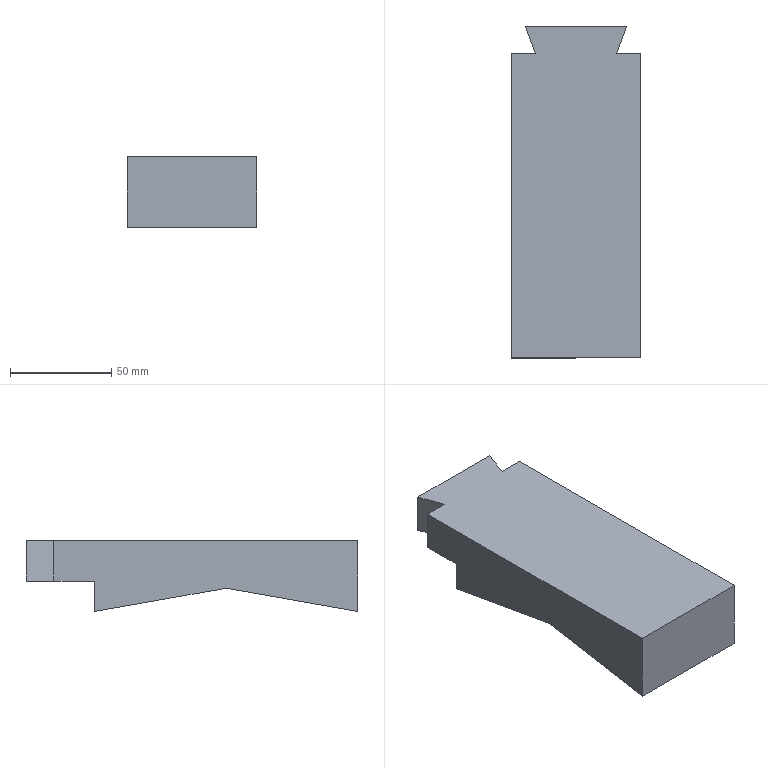Part | SolidWorks | features Extrusion 1, ICE 1 | 1 solid | 13 faces | box 64 x 163.737 x 35 mm | volume 281485 mm3 | plane 13
STEP:
#1=CARTESIAN_POINT('',(-27.262,-20.781,0.));
#2=VERTEX_POINT('',#1);
#3=CARTESIAN_POINT('',(36.738,-20.781,0.));
#4=VERTEX_POINT('',#3);
#5=CARTESIAN_POINT('',(-27.262,-20.781,0.));
#6=DIRECTION('',(1.,0.,0.));
#7=VECTOR('',#6,1000.);
#8=LINE('',#5,#7);
#9=EDGE_CURVE('',#2,#4,#8,.T.);
#10=ORIENTED_EDGE('',*,*,#9,.F.);
#11=CARTESIAN_POINT('',(-27.262,-0.7809,0.));
#12=VERTEX_POINT('',#11);
#13=CARTESIAN_POINT('',(-27.262,-0.7809,0.));
#14=DIRECTION('',(0.,-1.,0.));
#15=VECTOR('',#14,1000.);
#16=LINE('',#13,#15);
#17=EDGE_CURVE('',#12,#2,#16,.T.);
#18=ORIENTED_EDGE('',*,*,#17,.F.);
#19=CARTESIAN_POINT('',(-15.262,-0.7809,0.));
#20=VERTEX_POINT('',#19);
#21=CARTESIAN_POINT('',(-15.262,-0.7809,0.));
#22=DIRECTION('',(-1.,0.,0.));
#23=VECTOR('',#22,1000.);
#24=LINE('',#21,#23);
#25=EDGE_CURVE('',#20,#12,#24,.T.);
#26=ORIENTED_EDGE('',*,*,#25,.F.);
#27=CARTESIAN_POINT('',(-20.262,12.956,0.));
#28=VERTEX_POINT('',#27);
#29=CARTESIAN_POINT('',(-20.262,12.956,0.));
#30=DIRECTION('',(0.342,-0.9397,0.));
#31=VECTOR('',#30,1000.);
#32=LINE('',#29,#31);
#33=EDGE_CURVE('',#28,#20,#32,.T.);
#34=ORIENTED_EDGE('',*,*,#33,.F.);
#35=CARTESIAN_POINT('',(29.738,12.956,0.));
#36=VERTEX_POINT('',#35);
#37=CARTESIAN_POINT('',(29.738,12.956,0.));
#38=DIRECTION('',(-1.,0.,0.));
#39=VECTOR('',#38,1000.);
#40=LINE('',#37,#39);
#41=EDGE_CURVE('',#36,#28,#40,.T.);
#42=ORIENTED_EDGE('',*,*,#41,.F.);
#43=CARTESIAN_POINT('',(24.738,-0.7809,0.));
#44=VERTEX_POINT('',#43);
#45=CARTESIAN_POINT('',(24.738,-0.7809,0.));
#46=DIRECTION('',(0.342,0.9397,0.));
#47=VECTOR('',#46,1000.);
#48=LINE('',#45,#47);
#49=EDGE_CURVE('',#44,#36,#48,.T.);
#50=ORIENTED_EDGE('',*,*,#49,.F.);
#51=CARTESIAN_POINT('',(36.738,-0.7809,0.));
#52=VERTEX_POINT('',#51);
#53=CARTESIAN_POINT('',(36.738,-0.7809,0.));
#54=DIRECTION('',(-1.,0.,0.));
#55=VECTOR('',#54,1000.);
#56=LINE('',#53,#55);
#57=EDGE_CURVE('',#52,#44,#56,.T.);
#58=ORIENTED_EDGE('',*,*,#57,.F.);
#59=CARTESIAN_POINT('',(36.738,-0.7809,0.));
#60=DIRECTION('',(0.,1.,0.));
#61=VECTOR('',#60,1000.);
#62=LINE('',#59,#61);
#63=EDGE_CURVE('',#4,#52,#62,.T.);
#64=ORIENTED_EDGE('',*,*,#63,.F.);
#65=EDGE_LOOP('',(#10,#18,#26,#34,#42,#50,#58,#64));
#66=FACE_OUTER_BOUND('',#65,.T.);
#67=CARTESIAN_POINT('',(0.,0.,0.));
#68=DIRECTION('',(0.,0.,1.));
#69=DIRECTION('',(1.,0.,0.));
#70=AXIS2_PLACEMENT_3D('',#67,#68,#69);
#71=PLANE('',#70);
#72=ADVANCED_FACE('',(#66),#71,.F.);
#73=CARTESIAN_POINT('',(-27.262,-150.781,20.));
#74=VERTEX_POINT('',#73);
#75=CARTESIAN_POINT('',(-27.262,-150.781,-15.));
#76=VERTEX_POINT('',#75);
#77=CARTESIAN_POINT('',(-27.262,-150.781,20.));
#78=DIRECTION('',(0.,0.,-1.));
#79=VECTOR('',#78,1000.);
#80=LINE('',#77,#79);
#81=EDGE_CURVE('',#74,#76,#80,.T.);
#82=ORIENTED_EDGE('',*,*,#81,.T.);
#83=CARTESIAN_POINT('',(36.738,-150.781,-15.));
#84=VERTEX_POINT('',#83);
#85=CARTESIAN_POINT('',(-27.262,-150.781,-15.));
#86=DIRECTION('',(1.,0.,0.));
#87=VECTOR('',#86,1000.);
#88=LINE('',#85,#87);
#89=EDGE_CURVE('',#76,#84,#88,.T.);
#90=ORIENTED_EDGE('',*,*,#89,.T.);
#91=CARTESIAN_POINT('',(36.738,-150.781,20.));
#92=VERTEX_POINT('',#91);
#93=CARTESIAN_POINT('',(36.738,-150.781,20.));
#94=DIRECTION('',(0.,0.,-1.));
#95=VECTOR('',#94,1000.);
#96=LINE('',#93,#95);
#97=EDGE_CURVE('',#92,#84,#96,.T.);
#98=ORIENTED_EDGE('',*,*,#97,.F.);
#99=CARTESIAN_POINT('',(36.738,-150.781,20.));
#100=DIRECTION('',(1.,0.,0.));
#101=VECTOR('',#100,1000.);
#102=LINE('',#99,#101);
#103=EDGE_CURVE('',#74,#92,#102,.T.);
#104=ORIENTED_EDGE('',*,*,#103,.F.);
#105=EDGE_LOOP('',(#82,#90,#98,#104));
#106=FACE_OUTER_BOUND('',#105,.T.);
#107=CARTESIAN_POINT('',(36.738,-150.781,20.));
#108=DIRECTION('',(0.,1.,0.));
#109=DIRECTION('',(0.,0.,1.));
#110=AXIS2_PLACEMENT_3D('',#107,#108,#109);
#111=PLANE('',#110);
#112=ADVANCED_FACE('',(#106),#111,.F.);
#113=ORIENTED_EDGE('',*,*,#97,.T.);
#114=CARTESIAN_POINT('',(36.738,-85.784,-3.539));
#115=VERTEX_POINT('',#114);
#116=CARTESIAN_POINT('',(36.738,-150.781,-15.));
#117=DIRECTION('',(0.,0.9848,0.1737));
#118=VECTOR('',#117,1000.);
#119=LINE('',#116,#118);
#120=EDGE_CURVE('',#84,#115,#119,.T.);
#121=ORIENTED_EDGE('',*,*,#120,.T.);
#122=CARTESIAN_POINT('',(36.738,-20.781,-15.));
#123=VERTEX_POINT('',#122);
#124=CARTESIAN_POINT('',(36.738,-85.784,-3.539));
#125=DIRECTION('',(0.,0.9848,-0.1736));
#126=VECTOR('',#125,1000.);
#127=LINE('',#124,#126);
#128=EDGE_CURVE('',#115,#123,#127,.T.);
#129=ORIENTED_EDGE('',*,*,#128,.T.);
#130=CARTESIAN_POINT('',(36.738,-20.781,-15.));
#131=DIRECTION('',(0.,0.,1.));
#132=VECTOR('',#131,1000.);
#133=LINE('',#130,#132);
#134=EDGE_CURVE('',#123,#4,#133,.T.);
#135=ORIENTED_EDGE('',*,*,#134,.T.);
#136=ORIENTED_EDGE('',*,*,#63,.T.);
#137=CARTESIAN_POINT('',(36.738,-0.7809,20.));
#138=VERTEX_POINT('',#137);
#139=CARTESIAN_POINT('',(36.738,-0.7809,20.));
#140=DIRECTION('',(0.,0.,-1.));
#141=VECTOR('',#140,1000.);
#142=LINE('',#139,#141);
#143=EDGE_CURVE('',#138,#52,#142,.T.);
#144=ORIENTED_EDGE('',*,*,#143,.F.);
#145=CARTESIAN_POINT('',(36.738,-0.7809,20.));
#146=DIRECTION('',(0.,1.,0.));
#147=VECTOR('',#146,1000.);
#148=LINE('',#145,#147);
#149=EDGE_CURVE('',#92,#138,#148,.T.);
#150=ORIENTED_EDGE('',*,*,#149,.F.);
#151=EDGE_LOOP('',(#113,#121,#129,#135,#136,#144,#150));
#152=FACE_OUTER_BOUND('',#151,.T.);
#153=CARTESIAN_POINT('',(36.738,-0.7809,20.));
#154=DIRECTION('',(-1.,0.,0.));
#155=DIRECTION('',(0.,-1.,0.));
#156=AXIS2_PLACEMENT_3D('',#153,#154,#155);
#157=PLANE('',#156);
#158=ADVANCED_FACE('',(#152),#157,.F.);
#159=ORIENTED_EDGE('',*,*,#57,.T.);
#160=CARTESIAN_POINT('',(24.738,-0.7809,20.));
#161=VERTEX_POINT('',#160);
#162=CARTESIAN_POINT('',(24.738,-0.7809,20.));
#163=DIRECTION('',(0.,0.,-1.));
#164=VECTOR('',#163,1000.);
#165=LINE('',#162,#164);
#166=EDGE_CURVE('',#161,#44,#165,.T.);
#167=ORIENTED_EDGE('',*,*,#166,.F.);
#168=CARTESIAN_POINT('',(36.738,-0.7809,20.));
#169=DIRECTION('',(-1.,0.,0.));
#170=VECTOR('',#169,1000.);
#171=LINE('',#168,#170);
#172=EDGE_CURVE('',#138,#161,#171,.T.);
#173=ORIENTED_EDGE('',*,*,#172,.F.);
#174=ORIENTED_EDGE('',*,*,#143,.T.);
#175=EDGE_LOOP('',(#159,#167,#173,#174));
#176=FACE_OUTER_BOUND('',#175,.T.);
#177=CARTESIAN_POINT('',(36.738,-0.7809,20.));
#178=DIRECTION('',(0.,-1.,0.));
#179=DIRECTION('',(1.,0.,0.));
#180=AXIS2_PLACEMENT_3D('',#177,#178,#179);
#181=PLANE('',#180);
#182=ADVANCED_FACE('',(#176),#181,.F.);
#183=ORIENTED_EDGE('',*,*,#49,.T.);
#184=CARTESIAN_POINT('',(29.738,12.956,20.));
#185=VERTEX_POINT('',#184);
#186=CARTESIAN_POINT('',(29.738,12.956,20.));
#187=DIRECTION('',(0.,0.,-1.));
#188=VECTOR('',#187,1000.);
#189=LINE('',#186,#188);
#190=EDGE_CURVE('',#185,#36,#189,.T.);
#191=ORIENTED_EDGE('',*,*,#190,.F.);
#192=CARTESIAN_POINT('',(24.738,-0.7809,20.));
#193=DIRECTION('',(0.342,0.9397,0.));
#194=VECTOR('',#193,1000.);
#195=LINE('',#192,#194);
#196=EDGE_CURVE('',#161,#185,#195,.T.);
#197=ORIENTED_EDGE('',*,*,#196,.F.);
#198=ORIENTED_EDGE('',*,*,#166,.T.);
#199=EDGE_LOOP('',(#183,#191,#197,#198));
#200=FACE_OUTER_BOUND('',#199,.T.);
#201=CARTESIAN_POINT('',(24.738,-0.7809,20.));
#202=DIRECTION('',(-0.9397,0.342,0.));
#203=DIRECTION('',(-0.342,-0.9397,0.));
#204=AXIS2_PLACEMENT_3D('',#201,#202,#203);
#205=PLANE('',#204);
#206=ADVANCED_FACE('',(#200),#205,.F.);
#207=ORIENTED_EDGE('',*,*,#41,.T.);
#208=CARTESIAN_POINT('',(-20.262,12.956,20.));
#209=VERTEX_POINT('',#208);
#210=CARTESIAN_POINT('',(-20.262,12.956,20.));
#211=DIRECTION('',(0.,0.,-1.));
#212=VECTOR('',#211,1000.);
#213=LINE('',#210,#212);
#214=EDGE_CURVE('',#209,#28,#213,.T.);
#215=ORIENTED_EDGE('',*,*,#214,.F.);
#216=CARTESIAN_POINT('',(29.738,12.956,20.));
#217=DIRECTION('',(-1.,0.,0.));
#218=VECTOR('',#217,1000.);
#219=LINE('',#216,#218);
#220=EDGE_CURVE('',#185,#209,#219,.T.);
#221=ORIENTED_EDGE('',*,*,#220,.F.);
#222=ORIENTED_EDGE('',*,*,#190,.T.);
#223=EDGE_LOOP('',(#207,#215,#221,#222));
#224=FACE_OUTER_BOUND('',#223,.T.);
#225=CARTESIAN_POINT('',(29.738,12.956,20.));
#226=DIRECTION('',(0.,-1.,0.));
#227=DIRECTION('',(0.,0.,-1.));
#228=AXIS2_PLACEMENT_3D('',#225,#226,#227);
#229=PLANE('',#228);
#230=ADVANCED_FACE('',(#224),#229,.F.);
#231=ORIENTED_EDGE('',*,*,#33,.T.);
#232=CARTESIAN_POINT('',(-15.262,-0.7809,20.));
#233=VERTEX_POINT('',#232);
#234=CARTESIAN_POINT('',(-15.262,-0.7809,20.));
#235=DIRECTION('',(0.,0.,-1.));
#236=VECTOR('',#235,1000.);
#237=LINE('',#234,#236);
#238=EDGE_CURVE('',#233,#20,#237,.T.);
#239=ORIENTED_EDGE('',*,*,#238,.F.);
#240=CARTESIAN_POINT('',(-20.262,12.956,20.));
#241=DIRECTION('',(0.342,-0.9397,0.));
#242=VECTOR('',#241,1000.);
#243=LINE('',#240,#242);
#244=EDGE_CURVE('',#209,#233,#243,.T.);
#245=ORIENTED_EDGE('',*,*,#244,.F.);
#246=ORIENTED_EDGE('',*,*,#214,.T.);
#247=EDGE_LOOP('',(#231,#239,#245,#246));
#248=FACE_OUTER_BOUND('',#247,.T.);
#249=CARTESIAN_POINT('',(-20.262,12.956,20.));
#250=DIRECTION('',(0.9397,0.342,0.));
#251=DIRECTION('',(-0.342,0.9397,0.));
#252=AXIS2_PLACEMENT_3D('',#249,#250,#251);
#253=PLANE('',#252);
#254=ADVANCED_FACE('',(#248),#253,.F.);
#255=ORIENTED_EDGE('',*,*,#25,.T.);
#256=CARTESIAN_POINT('',(-27.262,-0.7809,20.));
#257=VERTEX_POINT('',#256);
#258=CARTESIAN_POINT('',(-27.262,-0.7809,20.));
#259=DIRECTION('',(0.,0.,-1.));
#260=VECTOR('',#259,1000.);
#261=LINE('',#258,#260);
#262=EDGE_CURVE('',#257,#12,#261,.T.);
#263=ORIENTED_EDGE('',*,*,#262,.F.);
#264=CARTESIAN_POINT('',(-15.262,-0.7809,20.));
#265=DIRECTION('',(-1.,0.,0.));
#266=VECTOR('',#265,1000.);
#267=LINE('',#264,#266);
#268=EDGE_CURVE('',#233,#257,#267,.T.);
#269=ORIENTED_EDGE('',*,*,#268,.F.);
#270=ORIENTED_EDGE('',*,*,#238,.T.);
#271=EDGE_LOOP('',(#255,#263,#269,#270));
#272=FACE_OUTER_BOUND('',#271,.T.);
#273=CARTESIAN_POINT('',(-15.262,-0.7809,20.));
#274=DIRECTION('',(0.,-1.,0.));
#275=DIRECTION('',(1.,0.,0.));
#276=AXIS2_PLACEMENT_3D('',#273,#274,#275);
#277=PLANE('',#276);
#278=ADVANCED_FACE('',(#272),#277,.F.);
#279=ORIENTED_EDGE('',*,*,#17,.T.);
#280=CARTESIAN_POINT('',(-27.262,-20.781,-15.));
#281=VERTEX_POINT('',#280);
#282=CARTESIAN_POINT('',(-27.262,-20.781,-15.));
#283=DIRECTION('',(0.,0.,1.));
#284=VECTOR('',#283,1000.);
#285=LINE('',#282,#284);
#286=EDGE_CURVE('',#281,#2,#285,.T.);
#287=ORIENTED_EDGE('',*,*,#286,.F.);
#288=CARTESIAN_POINT('',(-27.262,-85.784,-3.539));
#289=VERTEX_POINT('',#288);
#290=CARTESIAN_POINT('',(-27.262,-85.784,-3.539));
#291=DIRECTION('',(0.,0.9848,-0.1736));
#292=VECTOR('',#291,1000.);
#293=LINE('',#290,#292);
#294=EDGE_CURVE('',#289,#281,#293,.T.);
#295=ORIENTED_EDGE('',*,*,#294,.F.);
#296=CARTESIAN_POINT('',(-27.262,-150.781,-15.));
#297=DIRECTION('',(0.,0.9848,0.1737));
#298=VECTOR('',#297,1000.);
#299=LINE('',#296,#298);
#300=EDGE_CURVE('',#76,#289,#299,.T.);
#301=ORIENTED_EDGE('',*,*,#300,.F.);
#302=ORIENTED_EDGE('',*,*,#81,.F.);
#303=CARTESIAN_POINT('',(-27.262,-0.7809,20.));
#304=DIRECTION('',(0.,-1.,0.));
#305=VECTOR('',#304,1000.);
#306=LINE('',#303,#305);
#307=EDGE_CURVE('',#257,#74,#306,.T.);
#308=ORIENTED_EDGE('',*,*,#307,.F.);
#309=ORIENTED_EDGE('',*,*,#262,.T.);
#310=EDGE_LOOP('',(#279,#287,#295,#301,#302,#308,#309));
#311=FACE_OUTER_BOUND('',#310,.T.);
#312=CARTESIAN_POINT('',(-27.262,-0.7809,20.));
#313=DIRECTION('',(1.,0.,0.));
#314=DIRECTION('',(0.,1.,0.));
#315=AXIS2_PLACEMENT_3D('',#312,#313,#314);
#316=PLANE('',#315);
#317=ADVANCED_FACE('',(#311),#316,.F.);
#318=ORIENTED_EDGE('',*,*,#103,.T.);
#319=ORIENTED_EDGE('',*,*,#149,.T.);
#320=ORIENTED_EDGE('',*,*,#172,.T.);
#321=ORIENTED_EDGE('',*,*,#196,.T.);
#322=ORIENTED_EDGE('',*,*,#220,.T.);
#323=ORIENTED_EDGE('',*,*,#244,.T.);
#324=ORIENTED_EDGE('',*,*,#268,.T.);
#325=ORIENTED_EDGE('',*,*,#307,.T.);
#326=EDGE_LOOP('',(#318,#319,#320,#321,#322,#323,#324,#325));
#327=FACE_OUTER_BOUND('',#326,.T.);
#328=CARTESIAN_POINT('',(0.,0.,20.));
#329=DIRECTION('',(0.,0.,1.));
#330=DIRECTION('',(1.,0.,0.));
#331=AXIS2_PLACEMENT_3D('',#328,#329,#330);
#332=PLANE('',#331);
#333=ADVANCED_FACE('',(#327),#332,.T.);
#334=ORIENTED_EDGE('',*,*,#134,.F.);
#335=CARTESIAN_POINT('',(-27.262,-20.781,-15.));
#336=DIRECTION('',(1.,0.,0.));
#337=VECTOR('',#336,1000.);
#338=LINE('',#335,#337);
#339=EDGE_CURVE('',#281,#123,#338,.T.);
#340=ORIENTED_EDGE('',*,*,#339,.F.);
#341=ORIENTED_EDGE('',*,*,#286,.T.);
#342=ORIENTED_EDGE('',*,*,#9,.T.);
#343=EDGE_LOOP('',(#334,#340,#341,#342));
#344=FACE_OUTER_BOUND('',#343,.T.);
#345=CARTESIAN_POINT('',(-27.262,-20.781,-15.));
#346=DIRECTION('',(0.,1.,0.));
#347=DIRECTION('',(0.,0.,1.));
#348=AXIS2_PLACEMENT_3D('',#345,#346,#347);
#349=PLANE('',#348);
#350=ADVANCED_FACE('',(#344),#349,.T.);
#351=ORIENTED_EDGE('',*,*,#128,.F.);
#352=CARTESIAN_POINT('',(-27.262,-85.784,-3.539));
#353=DIRECTION('',(1.,0.,0.));
#354=VECTOR('',#353,1000.);
#355=LINE('',#352,#354);
#356=EDGE_CURVE('',#289,#115,#355,.T.);
#357=ORIENTED_EDGE('',*,*,#356,.F.);
#358=ORIENTED_EDGE('',*,*,#294,.T.);
#359=ORIENTED_EDGE('',*,*,#339,.T.);
#360=EDGE_LOOP('',(#351,#357,#358,#359));
#361=FACE_OUTER_BOUND('',#360,.T.);
#362=CARTESIAN_POINT('',(-27.262,-85.784,-3.539));
#363=DIRECTION('',(0.,-0.1736,-0.9848));
#364=DIRECTION('',(0.,0.9848,-0.1736));
#365=AXIS2_PLACEMENT_3D('',#362,#363,#364);
#366=PLANE('',#365);
#367=ADVANCED_FACE('',(#361),#366,.T.);
#368=ORIENTED_EDGE('',*,*,#120,.F.);
#369=ORIENTED_EDGE('',*,*,#89,.F.);
#370=ORIENTED_EDGE('',*,*,#300,.T.);
#371=ORIENTED_EDGE('',*,*,#356,.T.);
#372=EDGE_LOOP('',(#368,#369,#370,#371));
#373=FACE_OUTER_BOUND('',#372,.T.);
#374=CARTESIAN_POINT('',(-27.262,-150.781,-15.));
#375=DIRECTION('',(0.,0.1737,-0.9848));
#376=DIRECTION('',(0.,0.9848,0.1737));
#377=AXIS2_PLACEMENT_3D('',#374,#375,#376);
#378=PLANE('',#377);
#379=ADVANCED_FACE('',(#373),#378,.T.);
#380=CLOSED_SHELL('',(#72,#112,#158,#182,#206,#230,#254,#278,#317,#333,#350,#367,#379));
#381=MANIFOLD_SOLID_BREP('',#380);
#382=CARTESIAN_POINT('',(0.,0.,0.));
#383=DIRECTION('',(0.,0.,1.));
#384=DIRECTION('',(1.,0.,0.));
#385=AXIS2_PLACEMENT_3D('',#382,#383,#384);
#386=(LENGTH_UNIT()NAMED_UNIT(*)SI_UNIT(.MILLI.,.METRE.));
#387=UNCERTAINTY_MEASURE_WITH_UNIT(LENGTH_MEASURE(0.00001),#386,'','');
#388=(NAMED_UNIT(*)PLANE_ANGLE_UNIT()SI_UNIT($,.RADIAN.));
#389=(NAMED_UNIT(*)SI_UNIT($,.STERADIAN.)SOLID_ANGLE_UNIT());
#390=(GEOMETRIC_REPRESENTATION_CONTEXT(3)GLOBAL_UNCERTAINTY_ASSIGNED_CONTEXT((#387))GLOBAL_UNIT_ASSIGNED_CONTEXT((#386,#388,#389))REPRESENTATION_CONTEXT('',''));
#391=ADVANCED_BREP_SHAPE_REPRESENTATION('',(#381,#385),#390);